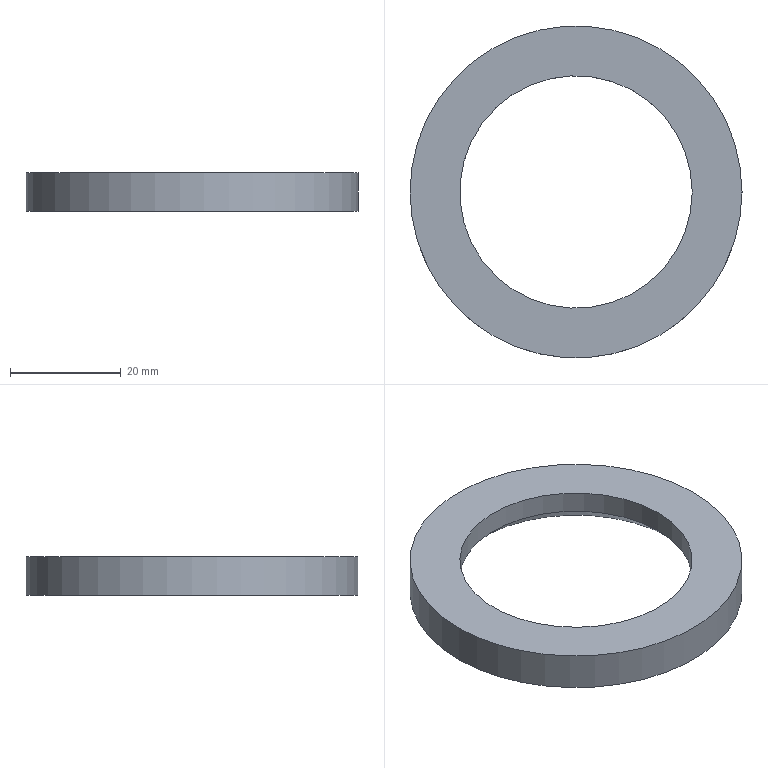Part | NX | features solid 2 | 1 solid | 5 faces | box 60 x 60 x 7 mm | volume 9472 mm3 | cylinder 2 | plane 2 | cone 1 | commonest cylinder face diameters 42 x1 60 x1
STEP:
#1=CARTESIAN_POINT('',(30.,0.,7.));
#2=VERTEX_POINT('',#1);
#3=CARTESIAN_POINT('',(0.,0.,7.));
#4=DIRECTION('',(0.,0.,1.));
#5=DIRECTION('',(1.,0.,0.));
#6=AXIS2_PLACEMENT_3D('',#3,#4,#5);
#7=CIRCLE('',#6,30.);
#8=EDGE_CURVE('',#2,#2,#7,.T.);
#9=ORIENTED_EDGE('',*,*,#8,.F.);
#10=EDGE_LOOP('',(#9));
#11=FACE_BOUND('',#10,.T.);
#12=CARTESIAN_POINT('',(30.,0.,0.));
#13=VERTEX_POINT('',#12);
#14=CARTESIAN_POINT('',(0.,0.,0.));
#15=DIRECTION('',(0.,0.,1.));
#16=DIRECTION('',(1.,0.,0.));
#17=AXIS2_PLACEMENT_3D('',#14,#15,#16);
#18=CIRCLE('',#17,30.);
#19=EDGE_CURVE('',#13,#13,#18,.T.);
#20=ORIENTED_EDGE('',*,*,#19,.T.);
#21=EDGE_LOOP('',(#20));
#22=FACE_BOUND('',#21,.T.);
#23=CARTESIAN_POINT('',(0.,0.,7.));
#24=DIRECTION('',(0.,0.,-1.));
#25=DIRECTION('',(-1.,0.,0.));
#26=AXIS2_PLACEMENT_3D('',#23,#24,#25);
#27=CYLINDRICAL_SURFACE('',#26,30.);
#28=ADVANCED_FACE('',(#11,#22),#27,.T.);
#29=CARTESIAN_POINT('',(21.,0.,3.));
#30=VERTEX_POINT('',#29);
#31=CARTESIAN_POINT('',(0.,0.,3.));
#32=DIRECTION('',(0.,0.,1.));
#33=DIRECTION('',(1.,0.,0.));
#34=AXIS2_PLACEMENT_3D('',#31,#32,#33);
#35=CIRCLE('',#34,21.);
#36=EDGE_CURVE('',#30,#30,#35,.F.);
#37=ORIENTED_EDGE('',*,*,#36,.T.);
#38=EDGE_LOOP('',(#37));
#39=FACE_BOUND('',#38,.T.);
#40=CARTESIAN_POINT('',(21.,0.,7.));
#41=VERTEX_POINT('',#40);
#42=CARTESIAN_POINT('',(0.,0.,7.));
#43=DIRECTION('',(0.,0.,1.));
#44=DIRECTION('',(1.,0.,0.));
#45=AXIS2_PLACEMENT_3D('',#42,#43,#44);
#46=CIRCLE('',#45,21.);
#47=EDGE_CURVE('',#41,#41,#46,.T.);
#48=ORIENTED_EDGE('',*,*,#47,.T.);
#49=EDGE_LOOP('',(#48));
#50=FACE_BOUND('',#49,.T.);
#51=CARTESIAN_POINT('',(0.,0.,7.));
#52=DIRECTION('',(0.,0.,-1.));
#53=DIRECTION('',(-1.,0.,0.));
#54=AXIS2_PLACEMENT_3D('',#51,#52,#53);
#55=CYLINDRICAL_SURFACE('',#54,21.);
#56=ADVANCED_FACE('',(#39,#50),#55,.F.);
#57=ORIENTED_EDGE('',*,*,#8,.T.);
#58=EDGE_LOOP('',(#57));
#59=FACE_BOUND('',#58,.T.);
#60=ORIENTED_EDGE('',*,*,#47,.F.);
#61=EDGE_LOOP('',(#60));
#62=FACE_BOUND('',#61,.T.);
#63=CARTESIAN_POINT('',(0.,0.,7.));
#64=DIRECTION('',(0.,0.,1.));
#65=DIRECTION('',(1.,0.,0.));
#66=AXIS2_PLACEMENT_3D('',#63,#64,#65);
#67=PLANE('',#66);
#68=ADVANCED_FACE('',(#59,#62),#67,.T.);
#69=CARTESIAN_POINT('',(24.,0.,0.));
#70=VERTEX_POINT('',#69);
#71=CARTESIAN_POINT('',(0.,0.,0.));
#72=DIRECTION('',(0.,0.,1.));
#73=DIRECTION('',(1.,0.,0.));
#74=AXIS2_PLACEMENT_3D('',#71,#72,#73);
#75=CIRCLE('',#74,24.);
#76=EDGE_CURVE('',#70,#70,#75,.T.);
#77=ORIENTED_EDGE('',*,*,#76,.T.);
#78=EDGE_LOOP('',(#77));
#79=FACE_BOUND('',#78,.T.);
#80=ORIENTED_EDGE('',*,*,#19,.F.);
#81=EDGE_LOOP('',(#80));
#82=FACE_BOUND('',#81,.T.);
#83=CARTESIAN_POINT('',(0.,0.,0.));
#84=DIRECTION('',(0.,0.,1.));
#85=DIRECTION('',(1.,0.,0.));
#86=AXIS2_PLACEMENT_3D('',#83,#84,#85);
#87=PLANE('',#86);
#88=ADVANCED_FACE('',(#79,#82),#87,.F.);
#89=ORIENTED_EDGE('',*,*,#36,.F.);
#90=EDGE_LOOP('',(#89));
#91=FACE_BOUND('',#90,.T.);
#92=ORIENTED_EDGE('',*,*,#76,.F.);
#93=EDGE_LOOP('',(#92));
#94=FACE_BOUND('',#93,.T.);
#95=CARTESIAN_POINT('',(0.,0.,0.));
#96=DIRECTION('',(0.,0.,-1.));
#97=DIRECTION('',(-1.,0.,0.));
#98=AXIS2_PLACEMENT_3D('',#95,#96,#97);
#99=CONICAL_SURFACE('',#98,24.,0.7854);
#100=ADVANCED_FACE('',(#91,#94),#99,.F.);
#101=CLOSED_SHELL('',(#28,#56,#68,#88,#100));
#102=MANIFOLD_SOLID_BREP('',#101);
#103=(LENGTH_UNIT()NAMED_UNIT(*)SI_UNIT(.MILLI.,.METRE.));
#104=UNCERTAINTY_MEASURE_WITH_UNIT(LENGTH_MEASURE(0.00001),#103,'','');
#105=(NAMED_UNIT(*)PLANE_ANGLE_UNIT()SI_UNIT($,.RADIAN.));
#106=(NAMED_UNIT(*)SI_UNIT($,.STERADIAN.)SOLID_ANGLE_UNIT());
#107=(GEOMETRIC_REPRESENTATION_CONTEXT(3)GLOBAL_UNCERTAINTY_ASSIGNED_CONTEXT((#104))GLOBAL_UNIT_ASSIGNED_CONTEXT((#103,#105,#106))REPRESENTATION_CONTEXT('',''));
#108=ADVANCED_BREP_SHAPE_REPRESENTATION('',(#102),#107);